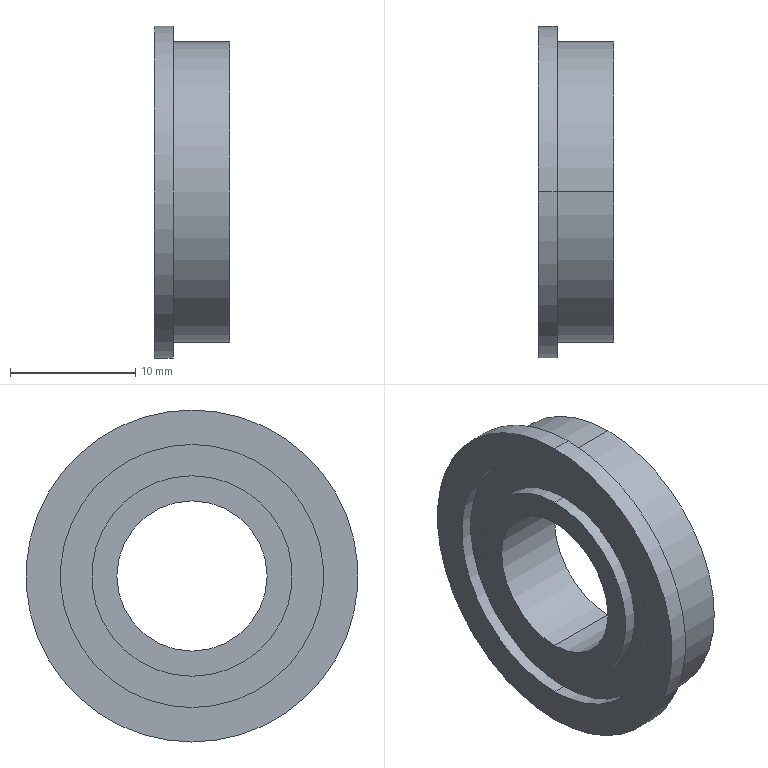Part | SolidWorks | features ICE 2, Revolution 1 | 1 solid | 21 faces | box 6 x 26.5 x 26.5 mm | volume 1894 mm3 | cylinder 14 | plane 7 | commonest cylinder face diameters 16 x4 21 x4 12 x2 24 x2 26.5 x2
STEP:
#1=CARTESIAN_POINT('',(1.,0.,8.));
#2=VERTEX_POINT('',#1);
#3=CARTESIAN_POINT('',(1.,0.,-8.));
#4=VERTEX_POINT('',#3);
#5=CARTESIAN_POINT('',(1.,0.,0.));
#6=DIRECTION('',(-1.,0.,0.));
#7=DIRECTION('',(0.,0.,1.));
#8=AXIS2_PLACEMENT_3D('',#5,#6,#7);
#9=CIRCLE('',#8,8.);
#10=EDGE_CURVE('',#2,#4,#9,.T.);
#11=ORIENTED_EDGE('',*,*,#10,.T.);
#12=CARTESIAN_POINT('',(0.,0.,-8.));
#13=VERTEX_POINT('',#12);
#14=CARTESIAN_POINT('',(1.,0.,-8.));
#15=DIRECTION('',(-1.,0.,0.));
#16=VECTOR('',#15,1000.);
#17=LINE('',#14,#16);
#18=EDGE_CURVE('',#4,#13,#17,.T.);
#19=ORIENTED_EDGE('',*,*,#18,.T.);
#20=CARTESIAN_POINT('',(0.,0.,8.));
#21=VERTEX_POINT('',#20);
#22=CARTESIAN_POINT('',(0.,0.,0.));
#23=DIRECTION('',(-1.,0.,0.));
#24=DIRECTION('',(0.,0.,1.));
#25=AXIS2_PLACEMENT_3D('',#22,#23,#24);
#26=CIRCLE('',#25,8.);
#27=EDGE_CURVE('',#21,#13,#26,.T.);
#28=ORIENTED_EDGE('',*,*,#27,.F.);
#29=CARTESIAN_POINT('',(1.,0.,8.));
#30=DIRECTION('',(-1.,0.,0.));
#31=VECTOR('',#30,1000.);
#32=LINE('',#29,#31);
#33=EDGE_CURVE('',#2,#21,#32,.T.);
#34=ORIENTED_EDGE('',*,*,#33,.F.);
#35=EDGE_LOOP('',(#11,#19,#28,#34));
#36=FACE_OUTER_BOUND('',#35,.T.);
#37=CARTESIAN_POINT('',(1.,0.,0.));
#38=DIRECTION('',(-1.,0.,0.));
#39=DIRECTION('',(0.,0.,1.));
#40=AXIS2_PLACEMENT_3D('',#37,#38,#39);
#41=CYLINDRICAL_SURFACE('',#40,8.);
#42=ADVANCED_FACE('',(#36),#41,.T.);
#43=CARTESIAN_POINT('',(1.,0.,-10.5));
#44=VERTEX_POINT('',#43);
#45=CARTESIAN_POINT('',(1.,0.,10.5));
#46=VERTEX_POINT('',#45);
#47=CARTESIAN_POINT('',(1.,0.,0.));
#48=DIRECTION('',(-1.,0.,0.));
#49=DIRECTION('',(0.,0.,1.));
#50=AXIS2_PLACEMENT_3D('',#47,#48,#49);
#51=CIRCLE('',#50,10.5);
#52=EDGE_CURVE('',#44,#46,#51,.T.);
#53=ORIENTED_EDGE('',*,*,#52,.F.);
#54=CARTESIAN_POINT('',(0.,0.,-10.5));
#55=VERTEX_POINT('',#54);
#56=CARTESIAN_POINT('',(1.,0.,-10.5));
#57=DIRECTION('',(-1.,0.,0.));
#58=VECTOR('',#57,1000.);
#59=LINE('',#56,#58);
#60=EDGE_CURVE('',#44,#55,#59,.T.);
#61=ORIENTED_EDGE('',*,*,#60,.T.);
#62=CARTESIAN_POINT('',(0.,0.,10.5));
#63=VERTEX_POINT('',#62);
#64=CARTESIAN_POINT('',(0.,0.,0.));
#65=DIRECTION('',(-1.,0.,0.));
#66=DIRECTION('',(0.,0.,1.));
#67=AXIS2_PLACEMENT_3D('',#64,#65,#66);
#68=CIRCLE('',#67,10.5);
#69=EDGE_CURVE('',#55,#63,#68,.T.);
#70=ORIENTED_EDGE('',*,*,#69,.T.);
#71=CARTESIAN_POINT('',(1.,0.,10.5));
#72=DIRECTION('',(-1.,0.,0.));
#73=VECTOR('',#72,1000.);
#74=LINE('',#71,#73);
#75=EDGE_CURVE('',#46,#63,#74,.T.);
#76=ORIENTED_EDGE('',*,*,#75,.F.);
#77=EDGE_LOOP('',(#53,#61,#70,#76));
#78=FACE_OUTER_BOUND('',#77,.T.);
#79=CARTESIAN_POINT('',(1.,0.,0.));
#80=DIRECTION('',(-1.,0.,0.));
#81=DIRECTION('',(0.,0.,1.));
#82=AXIS2_PLACEMENT_3D('',#79,#80,#81);
#83=CYLINDRICAL_SURFACE('',#82,10.5);
#84=ADVANCED_FACE('',(#78),#83,.F.);
#85=CARTESIAN_POINT('',(5.,0.,-8.));
#86=VERTEX_POINT('',#85);
#87=CARTESIAN_POINT('',(5.,0.,8.));
#88=VERTEX_POINT('',#87);
#89=CARTESIAN_POINT('',(5.,0.,0.));
#90=DIRECTION('',(1.,0.,0.));
#91=DIRECTION('',(0.,0.,-1.));
#92=AXIS2_PLACEMENT_3D('',#89,#90,#91);
#93=CIRCLE('',#92,8.);
#94=EDGE_CURVE('',#86,#88,#93,.T.);
#95=ORIENTED_EDGE('',*,*,#94,.T.);
#96=CARTESIAN_POINT('',(6.,0.,8.));
#97=VERTEX_POINT('',#96);
#98=CARTESIAN_POINT('',(5.,0.,8.));
#99=DIRECTION('',(1.,0.,0.));
#100=VECTOR('',#99,1000.);
#101=LINE('',#98,#100);
#102=EDGE_CURVE('',#88,#97,#101,.T.);
#103=ORIENTED_EDGE('',*,*,#102,.T.);
#104=CARTESIAN_POINT('',(6.,0.,-8.));
#105=VERTEX_POINT('',#104);
#106=CARTESIAN_POINT('',(6.,0.,0.));
#107=DIRECTION('',(1.,0.,0.));
#108=DIRECTION('',(0.,0.,-1.));
#109=AXIS2_PLACEMENT_3D('',#106,#107,#108);
#110=CIRCLE('',#109,8.);
#111=EDGE_CURVE('',#105,#97,#110,.T.);
#112=ORIENTED_EDGE('',*,*,#111,.F.);
#113=CARTESIAN_POINT('',(5.,0.,-8.));
#114=DIRECTION('',(1.,0.,0.));
#115=VECTOR('',#114,1000.);
#116=LINE('',#113,#115);
#117=EDGE_CURVE('',#86,#105,#116,.T.);
#118=ORIENTED_EDGE('',*,*,#117,.F.);
#119=EDGE_LOOP('',(#95,#103,#112,#118));
#120=FACE_OUTER_BOUND('',#119,.T.);
#121=CARTESIAN_POINT('',(5.,0.,0.));
#122=DIRECTION('',(1.,0.,0.));
#123=DIRECTION('',(0.,0.,-1.));
#124=AXIS2_PLACEMENT_3D('',#121,#122,#123);
#125=CYLINDRICAL_SURFACE('',#124,8.);
#126=ADVANCED_FACE('',(#120),#125,.T.);
#127=CARTESIAN_POINT('',(5.,0.,10.5));
#128=VERTEX_POINT('',#127);
#129=CARTESIAN_POINT('',(5.,0.,-10.5));
#130=VERTEX_POINT('',#129);
#131=CARTESIAN_POINT('',(5.,0.,0.));
#132=DIRECTION('',(1.,0.,0.));
#133=DIRECTION('',(0.,0.,-1.));
#134=AXIS2_PLACEMENT_3D('',#131,#132,#133);
#135=CIRCLE('',#134,10.5);
#136=EDGE_CURVE('',#128,#130,#135,.T.);
#137=ORIENTED_EDGE('',*,*,#136,.F.);
#138=CARTESIAN_POINT('',(6.,0.,10.5));
#139=VERTEX_POINT('',#138);
#140=CARTESIAN_POINT('',(5.,0.,10.5));
#141=DIRECTION('',(1.,0.,0.));
#142=VECTOR('',#141,1000.);
#143=LINE('',#140,#142);
#144=EDGE_CURVE('',#128,#139,#143,.T.);
#145=ORIENTED_EDGE('',*,*,#144,.T.);
#146=CARTESIAN_POINT('',(6.,0.,-10.5));
#147=VERTEX_POINT('',#146);
#148=CARTESIAN_POINT('',(6.,0.,0.));
#149=DIRECTION('',(1.,0.,0.));
#150=DIRECTION('',(0.,0.,-1.));
#151=AXIS2_PLACEMENT_3D('',#148,#149,#150);
#152=CIRCLE('',#151,10.5);
#153=EDGE_CURVE('',#139,#147,#152,.T.);
#154=ORIENTED_EDGE('',*,*,#153,.T.);
#155=CARTESIAN_POINT('',(5.,0.,-10.5));
#156=DIRECTION('',(1.,0.,0.));
#157=VECTOR('',#156,1000.);
#158=LINE('',#155,#157);
#159=EDGE_CURVE('',#130,#147,#158,.T.);
#160=ORIENTED_EDGE('',*,*,#159,.F.);
#161=EDGE_LOOP('',(#137,#145,#154,#160));
#162=FACE_OUTER_BOUND('',#161,.T.);
#163=CARTESIAN_POINT('',(5.,0.,0.));
#164=DIRECTION('',(1.,0.,0.));
#165=DIRECTION('',(0.,0.,-1.));
#166=AXIS2_PLACEMENT_3D('',#163,#164,#165);
#167=CYLINDRICAL_SURFACE('',#166,10.5);
#168=ADVANCED_FACE('',(#162),#167,.F.);
#169=CARTESIAN_POINT('',(1.5,0.,13.25));
#170=VERTEX_POINT('',#169);
#171=CARTESIAN_POINT('',(1.5,0.,-13.25));
#172=VERTEX_POINT('',#171);
#173=CARTESIAN_POINT('',(1.5,0.,0.));
#174=DIRECTION('',(-1.,0.,0.));
#175=DIRECTION('',(0.,0.,1.));
#176=AXIS2_PLACEMENT_3D('',#173,#174,#175);
#177=CIRCLE('',#176,13.25);
#178=EDGE_CURVE('',#170,#172,#177,.T.);
#179=ORIENTED_EDGE('',*,*,#178,.T.);
#180=CARTESIAN_POINT('',(0.,0.,-13.25));
#181=VERTEX_POINT('',#180);
#182=CARTESIAN_POINT('',(0.,0.,-13.25));
#183=DIRECTION('',(-1.,0.,0.));
#184=VECTOR('',#183,1000.);
#185=LINE('',#182,#184);
#186=EDGE_CURVE('',#172,#181,#185,.T.);
#187=ORIENTED_EDGE('',*,*,#186,.T.);
#188=CARTESIAN_POINT('',(0.,0.,13.25));
#189=VERTEX_POINT('',#188);
#190=CARTESIAN_POINT('',(0.,0.,0.));
#191=DIRECTION('',(-1.,0.,0.));
#192=DIRECTION('',(0.,0.,1.));
#193=AXIS2_PLACEMENT_3D('',#190,#191,#192);
#194=CIRCLE('',#193,13.25);
#195=EDGE_CURVE('',#189,#181,#194,.T.);
#196=ORIENTED_EDGE('',*,*,#195,.F.);
#197=CARTESIAN_POINT('',(0.,0.,13.25));
#198=DIRECTION('',(-1.,0.,0.));
#199=VECTOR('',#198,1000.);
#200=LINE('',#197,#199);
#201=EDGE_CURVE('',#170,#189,#200,.T.);
#202=ORIENTED_EDGE('',*,*,#201,.F.);
#203=EDGE_LOOP('',(#179,#187,#196,#202));
#204=FACE_OUTER_BOUND('',#203,.T.);
#205=CARTESIAN_POINT('',(0.,0.,0.));
#206=DIRECTION('',(-1.,0.,0.));
#207=DIRECTION('',(0.,0.,1.));
#208=AXIS2_PLACEMENT_3D('',#205,#206,#207);
#209=CYLINDRICAL_SURFACE('',#208,13.25);
#210=ADVANCED_FACE('',(#204),#209,.T.);
#211=CARTESIAN_POINT('',(6.,0.,12.));
#212=VERTEX_POINT('',#211);
#213=CARTESIAN_POINT('',(6.,0.,-12.));
#214=VERTEX_POINT('',#213);
#215=CARTESIAN_POINT('',(6.,0.,0.));
#216=DIRECTION('',(-1.,0.,0.));
#217=DIRECTION('',(0.,0.,1.));
#218=AXIS2_PLACEMENT_3D('',#215,#216,#217);
#219=CIRCLE('',#218,12.);
#220=EDGE_CURVE('',#212,#214,#219,.T.);
#221=ORIENTED_EDGE('',*,*,#220,.T.);
#222=CARTESIAN_POINT('',(1.5,0.,-12.));
#223=VERTEX_POINT('',#222);
#224=CARTESIAN_POINT('',(0.,0.,-12.));
#225=DIRECTION('',(-1.,0.,0.));
#226=VECTOR('',#225,1000.);
#227=LINE('',#224,#226);
#228=EDGE_CURVE('',#214,#223,#227,.T.);
#229=ORIENTED_EDGE('',*,*,#228,.T.);
#230=CARTESIAN_POINT('',(1.5,0.,12.));
#231=VERTEX_POINT('',#230);
#232=CARTESIAN_POINT('',(1.5,0.,0.));
#233=DIRECTION('',(-1.,0.,0.));
#234=DIRECTION('',(0.,0.,1.));
#235=AXIS2_PLACEMENT_3D('',#232,#233,#234);
#236=CIRCLE('',#235,12.);
#237=EDGE_CURVE('',#231,#223,#236,.T.);
#238=ORIENTED_EDGE('',*,*,#237,.F.);
#239=CARTESIAN_POINT('',(0.,0.,12.));
#240=DIRECTION('',(-1.,0.,0.));
#241=VECTOR('',#240,1000.);
#242=LINE('',#239,#241);
#243=EDGE_CURVE('',#212,#231,#242,.T.);
#244=ORIENTED_EDGE('',*,*,#243,.F.);
#245=EDGE_LOOP('',(#221,#229,#238,#244));
#246=FACE_OUTER_BOUND('',#245,.T.);
#247=CARTESIAN_POINT('',(0.,0.,0.));
#248=DIRECTION('',(-1.,0.,0.));
#249=DIRECTION('',(0.,0.,1.));
#250=AXIS2_PLACEMENT_3D('',#247,#248,#249);
#251=CYLINDRICAL_SURFACE('',#250,12.);
#252=ADVANCED_FACE('',(#246),#251,.T.);
#253=CARTESIAN_POINT('',(6.,0.,-6.));
#254=VERTEX_POINT('',#253);
#255=CARTESIAN_POINT('',(6.,0.,6.));
#256=VERTEX_POINT('',#255);
#257=CARTESIAN_POINT('',(6.,0.,0.));
#258=DIRECTION('',(-1.,0.,0.));
#259=DIRECTION('',(0.,0.,1.));
#260=AXIS2_PLACEMENT_3D('',#257,#258,#259);
#261=CIRCLE('',#260,6.);
#262=EDGE_CURVE('',#254,#256,#261,.T.);
#263=ORIENTED_EDGE('',*,*,#262,.F.);
#264=CARTESIAN_POINT('',(0.,0.,-6.));
#265=VERTEX_POINT('',#264);
#266=CARTESIAN_POINT('',(0.,0.,-6.));
#267=DIRECTION('',(-1.,0.,0.));
#268=VECTOR('',#267,1000.);
#269=LINE('',#266,#268);
#270=EDGE_CURVE('',#254,#265,#269,.T.);
#271=ORIENTED_EDGE('',*,*,#270,.T.);
#272=CARTESIAN_POINT('',(0.,0.,6.));
#273=VERTEX_POINT('',#272);
#274=CARTESIAN_POINT('',(0.,0.,0.));
#275=DIRECTION('',(-1.,0.,0.));
#276=DIRECTION('',(0.,0.,1.));
#277=AXIS2_PLACEMENT_3D('',#274,#275,#276);
#278=CIRCLE('',#277,6.);
#279=EDGE_CURVE('',#265,#273,#278,.T.);
#280=ORIENTED_EDGE('',*,*,#279,.T.);
#281=CARTESIAN_POINT('',(0.,0.,6.));
#282=DIRECTION('',(-1.,0.,0.));
#283=VECTOR('',#282,1000.);
#284=LINE('',#281,#283);
#285=EDGE_CURVE('',#256,#273,#284,.T.);
#286=ORIENTED_EDGE('',*,*,#285,.F.);
#287=EDGE_LOOP('',(#263,#271,#280,#286));
#288=FACE_OUTER_BOUND('',#287,.T.);
#289=CARTESIAN_POINT('',(0.,0.,0.));
#290=DIRECTION('',(-1.,0.,0.));
#291=DIRECTION('',(0.,0.,1.));
#292=AXIS2_PLACEMENT_3D('',#289,#290,#291);
#293=CYLINDRICAL_SURFACE('',#292,6.);
#294=ADVANCED_FACE('',(#288),#293,.F.);
#295=CARTESIAN_POINT('',(0.,0.,0.));
#296=DIRECTION('',(-1.,0.,0.));
#297=DIRECTION('',(0.,0.,1.));
#298=AXIS2_PLACEMENT_3D('',#295,#296,#297);
#299=CIRCLE('',#298,6.);
#300=EDGE_CURVE('',#273,#265,#299,.T.);
#301=ORIENTED_EDGE('',*,*,#300,.F.);
#302=ORIENTED_EDGE('',*,*,#279,.F.);
#303=EDGE_LOOP('',(#301,#302));
#304=FACE_BOUND('',#303,.T.);
#305=ORIENTED_EDGE('',*,*,#27,.T.);
#306=CARTESIAN_POINT('',(0.,0.,0.));
#307=DIRECTION('',(-1.,0.,0.));
#308=DIRECTION('',(0.,0.,1.));
#309=AXIS2_PLACEMENT_3D('',#306,#307,#308);
#310=CIRCLE('',#309,8.);
#311=EDGE_CURVE('',#13,#21,#310,.T.);
#312=ORIENTED_EDGE('',*,*,#311,.T.);
#313=EDGE_LOOP('',(#305,#312));
#314=FACE_OUTER_BOUND('',#313,.T.);
#315=CARTESIAN_POINT('',(0.,0.,0.));
#316=DIRECTION('',(1.,0.,0.));
#317=DIRECTION('',(0.,0.,-1.));
#318=AXIS2_PLACEMENT_3D('',#315,#316,#317);
#319=PLANE('',#318);
#320=ADVANCED_FACE('',(#304,#314),#319,.F.);
#321=CARTESIAN_POINT('',(6.,0.,0.));
#322=DIRECTION('',(-1.,0.,0.));
#323=DIRECTION('',(0.,0.,1.));
#324=AXIS2_PLACEMENT_3D('',#321,#322,#323);
#325=CIRCLE('',#324,6.);
#326=EDGE_CURVE('',#256,#254,#325,.T.);
#327=ORIENTED_EDGE('',*,*,#326,.T.);
#328=ORIENTED_EDGE('',*,*,#262,.T.);
#329=EDGE_LOOP('',(#327,#328));
#330=FACE_BOUND('',#329,.T.);
#331=ORIENTED_EDGE('',*,*,#111,.T.);
#332=CARTESIAN_POINT('',(6.,0.,0.));
#333=DIRECTION('',(1.,0.,0.));
#334=DIRECTION('',(0.,0.,-1.));
#335=AXIS2_PLACEMENT_3D('',#332,#333,#334);
#336=CIRCLE('',#335,8.);
#337=EDGE_CURVE('',#97,#105,#336,.T.);
#338=ORIENTED_EDGE('',*,*,#337,.T.);
#339=EDGE_LOOP('',(#331,#338));
#340=FACE_OUTER_BOUND('',#339,.T.);
#341=CARTESIAN_POINT('',(6.,0.,0.));
#342=DIRECTION('',(-1.,0.,0.));
#343=DIRECTION('',(0.,0.,1.));
#344=AXIS2_PLACEMENT_3D('',#341,#342,#343);
#345=PLANE('',#344);
#346=ADVANCED_FACE('',(#330,#340),#345,.F.);
#347=CARTESIAN_POINT('',(0.,0.,0.));
#348=DIRECTION('',(-1.,0.,0.));
#349=DIRECTION('',(0.,0.,1.));
#350=AXIS2_PLACEMENT_3D('',#347,#348,#349);
#351=CIRCLE('',#350,10.5);
#352=EDGE_CURVE('',#63,#55,#351,.T.);
#353=ORIENTED_EDGE('',*,*,#352,.F.);
#354=ORIENTED_EDGE('',*,*,#69,.F.);
#355=EDGE_LOOP('',(#353,#354));
#356=FACE_BOUND('',#355,.T.);
#357=ORIENTED_EDGE('',*,*,#195,.T.);
#358=CARTESIAN_POINT('',(0.,0.,0.));
#359=DIRECTION('',(-1.,0.,0.));
#360=DIRECTION('',(0.,0.,1.));
#361=AXIS2_PLACEMENT_3D('',#358,#359,#360);
#362=CIRCLE('',#361,13.25);
#363=EDGE_CURVE('',#181,#189,#362,.T.);
#364=ORIENTED_EDGE('',*,*,#363,.T.);
#365=EDGE_LOOP('',(#357,#364));
#366=FACE_OUTER_BOUND('',#365,.T.);
#367=CARTESIAN_POINT('',(0.,0.,0.));
#368=DIRECTION('',(1.,0.,0.));
#369=DIRECTION('',(0.,0.,-1.));
#370=AXIS2_PLACEMENT_3D('',#367,#368,#369);
#371=PLANE('',#370);
#372=ADVANCED_FACE('',(#356,#366),#371,.F.);
#373=ORIENTED_EDGE('',*,*,#270,.F.);
#374=ORIENTED_EDGE('',*,*,#326,.F.);
#375=ORIENTED_EDGE('',*,*,#285,.T.);
#376=ORIENTED_EDGE('',*,*,#300,.T.);
#377=EDGE_LOOP('',(#373,#374,#375,#376));
#378=FACE_OUTER_BOUND('',#377,.T.);
#379=CARTESIAN_POINT('',(0.,0.,0.));
#380=DIRECTION('',(-1.,0.,0.));
#381=DIRECTION('',(0.,0.,1.));
#382=AXIS2_PLACEMENT_3D('',#379,#380,#381);
#383=CYLINDRICAL_SURFACE('',#382,6.);
#384=ADVANCED_FACE('',(#378),#383,.F.);
#385=CARTESIAN_POINT('',(6.,0.,0.));
#386=DIRECTION('',(1.,0.,0.));
#387=DIRECTION('',(0.,0.,-1.));
#388=AXIS2_PLACEMENT_3D('',#385,#386,#387);
#389=CIRCLE('',#388,10.5);
#390=EDGE_CURVE('',#147,#139,#389,.T.);
#391=ORIENTED_EDGE('',*,*,#390,.F.);
#392=ORIENTED_EDGE('',*,*,#153,.F.);
#393=EDGE_LOOP('',(#391,#392));
#394=FACE_BOUND('',#393,.T.);
#395=ORIENTED_EDGE('',*,*,#220,.F.);
#396=CARTESIAN_POINT('',(6.,0.,0.));
#397=DIRECTION('',(-1.,0.,0.));
#398=DIRECTION('',(0.,0.,1.));
#399=AXIS2_PLACEMENT_3D('',#396,#397,#398);
#400=CIRCLE('',#399,12.);
#401=EDGE_CURVE('',#214,#212,#400,.T.);
#402=ORIENTED_EDGE('',*,*,#401,.F.);
#403=EDGE_LOOP('',(#395,#402));
#404=FACE_OUTER_BOUND('',#403,.T.);
#405=CARTESIAN_POINT('',(6.,0.,0.));
#406=DIRECTION('',(-1.,0.,0.));
#407=DIRECTION('',(0.,0.,1.));
#408=AXIS2_PLACEMENT_3D('',#405,#406,#407);
#409=PLANE('',#408);
#410=ADVANCED_FACE('',(#394,#404),#409,.F.);
#411=ORIENTED_EDGE('',*,*,#228,.F.);
#412=ORIENTED_EDGE('',*,*,#401,.T.);
#413=ORIENTED_EDGE('',*,*,#243,.T.);
#414=CARTESIAN_POINT('',(1.5,0.,0.));
#415=DIRECTION('',(-1.,0.,0.));
#416=DIRECTION('',(0.,0.,1.));
#417=AXIS2_PLACEMENT_3D('',#414,#415,#416);
#418=CIRCLE('',#417,12.);
#419=EDGE_CURVE('',#223,#231,#418,.T.);
#420=ORIENTED_EDGE('',*,*,#419,.F.);
#421=EDGE_LOOP('',(#411,#412,#413,#420));
#422=FACE_OUTER_BOUND('',#421,.T.);
#423=CARTESIAN_POINT('',(0.,0.,0.));
#424=DIRECTION('',(-1.,0.,0.));
#425=DIRECTION('',(0.,0.,1.));
#426=AXIS2_PLACEMENT_3D('',#423,#424,#425);
#427=CYLINDRICAL_SURFACE('',#426,12.);
#428=ADVANCED_FACE('',(#422),#427,.T.);
#429=ORIENTED_EDGE('',*,*,#178,.F.);
#430=CARTESIAN_POINT('',(1.5,0.,0.));
#431=DIRECTION('',(-1.,0.,0.));
#432=DIRECTION('',(0.,0.,1.));
#433=AXIS2_PLACEMENT_3D('',#430,#431,#432);
#434=CIRCLE('',#433,13.25);
#435=EDGE_CURVE('',#172,#170,#434,.T.);
#436=ORIENTED_EDGE('',*,*,#435,.F.);
#437=EDGE_LOOP('',(#429,#436));
#438=FACE_OUTER_BOUND('',#437,.T.);
#439=ORIENTED_EDGE('',*,*,#237,.T.);
#440=ORIENTED_EDGE('',*,*,#419,.T.);
#441=EDGE_LOOP('',(#439,#440));
#442=FACE_BOUND('',#441,.T.);
#443=CARTESIAN_POINT('',(1.5,0.,0.));
#444=DIRECTION('',(-1.,0.,0.));
#445=DIRECTION('',(0.,0.,1.));
#446=AXIS2_PLACEMENT_3D('',#443,#444,#445);
#447=PLANE('',#446);
#448=ADVANCED_FACE('',(#438,#442),#447,.F.);
#449=ORIENTED_EDGE('',*,*,#186,.F.);
#450=ORIENTED_EDGE('',*,*,#435,.T.);
#451=ORIENTED_EDGE('',*,*,#201,.T.);
#452=ORIENTED_EDGE('',*,*,#363,.F.);
#453=EDGE_LOOP('',(#449,#450,#451,#452));
#454=FACE_OUTER_BOUND('',#453,.T.);
#455=CARTESIAN_POINT('',(0.,0.,0.));
#456=DIRECTION('',(-1.,0.,0.));
#457=DIRECTION('',(0.,0.,1.));
#458=AXIS2_PLACEMENT_3D('',#455,#456,#457);
#459=CYLINDRICAL_SURFACE('',#458,13.25);
#460=ADVANCED_FACE('',(#454),#459,.T.);
#461=ORIENTED_EDGE('',*,*,#144,.F.);
#462=CARTESIAN_POINT('',(5.,0.,0.));
#463=DIRECTION('',(1.,0.,0.));
#464=DIRECTION('',(0.,0.,-1.));
#465=AXIS2_PLACEMENT_3D('',#462,#463,#464);
#466=CIRCLE('',#465,10.5);
#467=EDGE_CURVE('',#130,#128,#466,.T.);
#468=ORIENTED_EDGE('',*,*,#467,.F.);
#469=ORIENTED_EDGE('',*,*,#159,.T.);
#470=ORIENTED_EDGE('',*,*,#390,.T.);
#471=EDGE_LOOP('',(#461,#468,#469,#470));
#472=FACE_OUTER_BOUND('',#471,.T.);
#473=CARTESIAN_POINT('',(5.,0.,0.));
#474=DIRECTION('',(1.,0.,0.));
#475=DIRECTION('',(0.,0.,-1.));
#476=AXIS2_PLACEMENT_3D('',#473,#474,#475);
#477=CYLINDRICAL_SURFACE('',#476,10.5);
#478=ADVANCED_FACE('',(#472),#477,.F.);
#479=ORIENTED_EDGE('',*,*,#94,.F.);
#480=CARTESIAN_POINT('',(5.,0.,0.));
#481=DIRECTION('',(1.,0.,0.));
#482=DIRECTION('',(0.,0.,-1.));
#483=AXIS2_PLACEMENT_3D('',#480,#481,#482);
#484=CIRCLE('',#483,8.);
#485=EDGE_CURVE('',#88,#86,#484,.T.);
#486=ORIENTED_EDGE('',*,*,#485,.F.);
#487=EDGE_LOOP('',(#479,#486));
#488=FACE_BOUND('',#487,.T.);
#489=ORIENTED_EDGE('',*,*,#467,.T.);
#490=ORIENTED_EDGE('',*,*,#136,.T.);
#491=EDGE_LOOP('',(#489,#490));
#492=FACE_OUTER_BOUND('',#491,.T.);
#493=CARTESIAN_POINT('',(5.,0.,0.));
#494=DIRECTION('',(1.,0.,0.));
#495=DIRECTION('',(0.,0.,-1.));
#496=AXIS2_PLACEMENT_3D('',#493,#494,#495);
#497=PLANE('',#496);
#498=ADVANCED_FACE('',(#488,#492),#497,.T.);
#499=ORIENTED_EDGE('',*,*,#102,.F.);
#500=ORIENTED_EDGE('',*,*,#485,.T.);
#501=ORIENTED_EDGE('',*,*,#117,.T.);
#502=ORIENTED_EDGE('',*,*,#337,.F.);
#503=EDGE_LOOP('',(#499,#500,#501,#502));
#504=FACE_OUTER_BOUND('',#503,.T.);
#505=CARTESIAN_POINT('',(5.,0.,0.));
#506=DIRECTION('',(1.,0.,0.));
#507=DIRECTION('',(0.,0.,-1.));
#508=AXIS2_PLACEMENT_3D('',#505,#506,#507);
#509=CYLINDRICAL_SURFACE('',#508,8.);
#510=ADVANCED_FACE('',(#504),#509,.T.);
#511=ORIENTED_EDGE('',*,*,#60,.F.);
#512=CARTESIAN_POINT('',(1.,0.,0.));
#513=DIRECTION('',(-1.,0.,0.));
#514=DIRECTION('',(0.,0.,1.));
#515=AXIS2_PLACEMENT_3D('',#512,#513,#514);
#516=CIRCLE('',#515,10.5);
#517=EDGE_CURVE('',#46,#44,#516,.T.);
#518=ORIENTED_EDGE('',*,*,#517,.F.);
#519=ORIENTED_EDGE('',*,*,#75,.T.);
#520=ORIENTED_EDGE('',*,*,#352,.T.);
#521=EDGE_LOOP('',(#511,#518,#519,#520));
#522=FACE_OUTER_BOUND('',#521,.T.);
#523=CARTESIAN_POINT('',(1.,0.,0.));
#524=DIRECTION('',(-1.,0.,0.));
#525=DIRECTION('',(0.,0.,1.));
#526=AXIS2_PLACEMENT_3D('',#523,#524,#525);
#527=CYLINDRICAL_SURFACE('',#526,10.5);
#528=ADVANCED_FACE('',(#522),#527,.F.);
#529=ORIENTED_EDGE('',*,*,#10,.F.);
#530=CARTESIAN_POINT('',(1.,0.,0.));
#531=DIRECTION('',(-1.,0.,0.));
#532=DIRECTION('',(0.,0.,1.));
#533=AXIS2_PLACEMENT_3D('',#530,#531,#532);
#534=CIRCLE('',#533,8.);
#535=EDGE_CURVE('',#4,#2,#534,.T.);
#536=ORIENTED_EDGE('',*,*,#535,.F.);
#537=EDGE_LOOP('',(#529,#536));
#538=FACE_BOUND('',#537,.T.);
#539=ORIENTED_EDGE('',*,*,#517,.T.);
#540=ORIENTED_EDGE('',*,*,#52,.T.);
#541=EDGE_LOOP('',(#539,#540));
#542=FACE_OUTER_BOUND('',#541,.T.);
#543=CARTESIAN_POINT('',(1.,0.,0.));
#544=DIRECTION('',(-1.,0.,0.));
#545=DIRECTION('',(0.,0.,1.));
#546=AXIS2_PLACEMENT_3D('',#543,#544,#545);
#547=PLANE('',#546);
#548=ADVANCED_FACE('',(#538,#542),#547,.T.);
#549=ORIENTED_EDGE('',*,*,#18,.F.);
#550=ORIENTED_EDGE('',*,*,#535,.T.);
#551=ORIENTED_EDGE('',*,*,#33,.T.);
#552=ORIENTED_EDGE('',*,*,#311,.F.);
#553=EDGE_LOOP('',(#549,#550,#551,#552));
#554=FACE_OUTER_BOUND('',#553,.T.);
#555=CARTESIAN_POINT('',(1.,0.,0.));
#556=DIRECTION('',(-1.,0.,0.));
#557=DIRECTION('',(0.,0.,1.));
#558=AXIS2_PLACEMENT_3D('',#555,#556,#557);
#559=CYLINDRICAL_SURFACE('',#558,8.);
#560=ADVANCED_FACE('',(#554),#559,.T.);
#561=CLOSED_SHELL('',(#42,#84,#126,#168,#210,#252,#294,#320,#346,#372,#384,#410,#428,#448,#460,#478,#498,#510,#528,#548,#560));
#562=MANIFOLD_SOLID_BREP('',#561);
#563=CARTESIAN_POINT('',(0.,0.,0.));
#564=DIRECTION('',(0.,0.,1.));
#565=DIRECTION('',(1.,0.,0.));
#566=AXIS2_PLACEMENT_3D('',#563,#564,#565);
#567=(LENGTH_UNIT()NAMED_UNIT(*)SI_UNIT(.MILLI.,.METRE.));
#568=UNCERTAINTY_MEASURE_WITH_UNIT(LENGTH_MEASURE(0.00001),#567,'','');
#569=(NAMED_UNIT(*)PLANE_ANGLE_UNIT()SI_UNIT($,.RADIAN.));
#570=(NAMED_UNIT(*)SI_UNIT($,.STERADIAN.)SOLID_ANGLE_UNIT());
#571=(GEOMETRIC_REPRESENTATION_CONTEXT(3)GLOBAL_UNCERTAINTY_ASSIGNED_CONTEXT((#568))GLOBAL_UNIT_ASSIGNED_CONTEXT((#567,#569,#570))REPRESENTATION_CONTEXT('',''));
#572=ADVANCED_BREP_SHAPE_REPRESENTATION('',(#562,#566),#571);